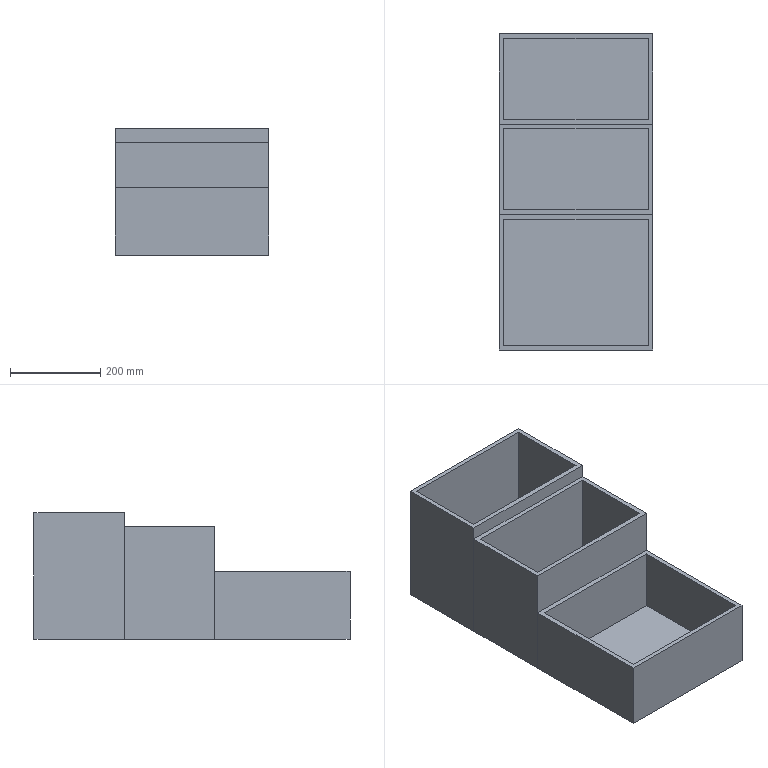Part | SolidWorks | features Shell 3, ICE 2, Extrusion 1 | 3 solids | 33 faces | box 340 x 700 x 280 mm | volume 9420000 mm3 | plane 33
STEP:
#1=CARTESIAN_POINT('',(170.,-100.,280.));
#2=VERTEX_POINT('',#1);
#3=CARTESIAN_POINT('',(170.,100.,280.));
#4=VERTEX_POINT('',#3);
#5=CARTESIAN_POINT('',(170.,-100.,280.));
#6=DIRECTION('',(0.,1.,0.));
#7=VECTOR('',#6,1000.);
#8=LINE('',#5,#7);
#9=EDGE_CURVE('',#2,#4,#8,.T.);
#10=ORIENTED_EDGE('',*,*,#9,.T.);
#11=CARTESIAN_POINT('',(-170.,100.,280.));
#12=VERTEX_POINT('',#11);
#13=CARTESIAN_POINT('',(-170.,100.,280.));
#14=DIRECTION('',(-1.,0.,0.));
#15=VECTOR('',#14,1000.);
#16=LINE('',#13,#15);
#17=EDGE_CURVE('',#4,#12,#16,.T.);
#18=ORIENTED_EDGE('',*,*,#17,.T.);
#19=CARTESIAN_POINT('',(-170.,-100.,280.));
#20=VERTEX_POINT('',#19);
#21=CARTESIAN_POINT('',(-170.,-100.,280.));
#22=DIRECTION('',(0.,-1.,0.));
#23=VECTOR('',#22,1000.);
#24=LINE('',#21,#23);
#25=EDGE_CURVE('',#12,#20,#24,.T.);
#26=ORIENTED_EDGE('',*,*,#25,.T.);
#27=CARTESIAN_POINT('',(-170.,-100.,280.));
#28=DIRECTION('',(1.,0.,0.));
#29=VECTOR('',#28,1000.);
#30=LINE('',#27,#29);
#31=EDGE_CURVE('',#20,#2,#30,.T.);
#32=ORIENTED_EDGE('',*,*,#31,.T.);
#33=EDGE_LOOP('',(#10,#18,#26,#32));
#34=FACE_OUTER_BOUND('',#33,.T.);
#35=CARTESIAN_POINT('',(160.,-90.,280.));
#36=VERTEX_POINT('',#35);
#37=CARTESIAN_POINT('',(160.,90.,280.));
#38=VERTEX_POINT('',#37);
#39=CARTESIAN_POINT('',(160.,0.,280.));
#40=DIRECTION('',(0.,1.,0.));
#41=VECTOR('',#40,1000.);
#42=LINE('',#39,#41);
#43=EDGE_CURVE('',#36,#38,#42,.T.);
#44=ORIENTED_EDGE('',*,*,#43,.F.);
#45=CARTESIAN_POINT('',(-160.,-90.,280.));
#46=VERTEX_POINT('',#45);
#47=CARTESIAN_POINT('',(0.,-90.,280.));
#48=DIRECTION('',(1.,0.,0.));
#49=VECTOR('',#48,1000.);
#50=LINE('',#47,#49);
#51=EDGE_CURVE('',#46,#36,#50,.T.);
#52=ORIENTED_EDGE('',*,*,#51,.F.);
#53=CARTESIAN_POINT('',(-160.,90.,280.));
#54=VERTEX_POINT('',#53);
#55=CARTESIAN_POINT('',(-160.,0.,280.));
#56=DIRECTION('',(0.,-1.,0.));
#57=VECTOR('',#56,1000.);
#58=LINE('',#55,#57);
#59=EDGE_CURVE('',#54,#46,#58,.T.);
#60=ORIENTED_EDGE('',*,*,#59,.F.);
#61=CARTESIAN_POINT('',(0.,90.,280.));
#62=DIRECTION('',(-1.,0.,0.));
#63=VECTOR('',#62,1000.);
#64=LINE('',#61,#63);
#65=EDGE_CURVE('',#38,#54,#64,.T.);
#66=ORIENTED_EDGE('',*,*,#65,.F.);
#67=EDGE_LOOP('',(#44,#52,#60,#66));
#68=FACE_BOUND('',#67,.T.);
#69=CARTESIAN_POINT('',(0.,0.,280.));
#70=DIRECTION('',(0.,0.,-1.));
#71=DIRECTION('',(-1.,0.,0.));
#72=AXIS2_PLACEMENT_3D('',#69,#70,#71);
#73=PLANE('',#72);
#74=ADVANCED_FACE('',(#34,#68),#73,.F.);
#75=CARTESIAN_POINT('',(170.,-100.,0.));
#76=VERTEX_POINT('',#75);
#77=CARTESIAN_POINT('',(170.,100.,0.));
#78=VERTEX_POINT('',#77);
#79=CARTESIAN_POINT('',(170.,-100.,0.));
#80=DIRECTION('',(0.,1.,0.));
#81=VECTOR('',#80,1000.);
#82=LINE('',#79,#81);
#83=EDGE_CURVE('',#76,#78,#82,.T.);
#84=ORIENTED_EDGE('',*,*,#83,.T.);
#85=CARTESIAN_POINT('',(170.,100.,280.));
#86=DIRECTION('',(0.,0.,-1.));
#87=VECTOR('',#86,1000.);
#88=LINE('',#85,#87);
#89=EDGE_CURVE('',#4,#78,#88,.T.);
#90=ORIENTED_EDGE('',*,*,#89,.F.);
#91=ORIENTED_EDGE('',*,*,#9,.F.);
#92=CARTESIAN_POINT('',(170.,-100.,280.));
#93=DIRECTION('',(0.,0.,-1.));
#94=VECTOR('',#93,1000.);
#95=LINE('',#92,#94);
#96=EDGE_CURVE('',#2,#76,#95,.T.);
#97=ORIENTED_EDGE('',*,*,#96,.T.);
#98=EDGE_LOOP('',(#84,#90,#91,#97));
#99=FACE_OUTER_BOUND('',#98,.T.);
#100=CARTESIAN_POINT('',(170.,-100.,280.));
#101=DIRECTION('',(-1.,0.,0.));
#102=DIRECTION('',(0.,0.,1.));
#103=AXIS2_PLACEMENT_3D('',#100,#101,#102);
#104=PLANE('',#103);
#105=ADVANCED_FACE('',(#99),#104,.F.);
#106=CARTESIAN_POINT('',(-170.,100.,0.));
#107=VERTEX_POINT('',#106);
#108=CARTESIAN_POINT('',(-170.,100.,0.));
#109=DIRECTION('',(-1.,0.,0.));
#110=VECTOR('',#109,1000.);
#111=LINE('',#108,#110);
#112=EDGE_CURVE('',#78,#107,#111,.T.);
#113=ORIENTED_EDGE('',*,*,#112,.T.);
#114=CARTESIAN_POINT('',(-170.,100.,280.));
#115=DIRECTION('',(0.,0.,-1.));
#116=VECTOR('',#115,1000.);
#117=LINE('',#114,#116);
#118=EDGE_CURVE('',#12,#107,#117,.T.);
#119=ORIENTED_EDGE('',*,*,#118,.F.);
#120=ORIENTED_EDGE('',*,*,#17,.F.);
#121=ORIENTED_EDGE('',*,*,#89,.T.);
#122=EDGE_LOOP('',(#113,#119,#120,#121));
#123=FACE_OUTER_BOUND('',#122,.T.);
#124=CARTESIAN_POINT('',(-170.,100.,280.));
#125=DIRECTION('',(0.,-1.,0.));
#126=DIRECTION('',(0.,0.,-1.));
#127=AXIS2_PLACEMENT_3D('',#124,#125,#126);
#128=PLANE('',#127);
#129=ADVANCED_FACE('',(#123),#128,.F.);
#130=CARTESIAN_POINT('',(-170.,-100.,0.));
#131=VERTEX_POINT('',#130);
#132=CARTESIAN_POINT('',(-170.,-100.,0.));
#133=DIRECTION('',(0.,-1.,0.));
#134=VECTOR('',#133,1000.);
#135=LINE('',#132,#134);
#136=EDGE_CURVE('',#107,#131,#135,.T.);
#137=ORIENTED_EDGE('',*,*,#136,.T.);
#138=CARTESIAN_POINT('',(-170.,-100.,280.));
#139=DIRECTION('',(0.,0.,-1.));
#140=VECTOR('',#139,1000.);
#141=LINE('',#138,#140);
#142=EDGE_CURVE('',#20,#131,#141,.T.);
#143=ORIENTED_EDGE('',*,*,#142,.F.);
#144=ORIENTED_EDGE('',*,*,#25,.F.);
#145=ORIENTED_EDGE('',*,*,#118,.T.);
#146=EDGE_LOOP('',(#137,#143,#144,#145));
#147=FACE_OUTER_BOUND('',#146,.T.);
#148=CARTESIAN_POINT('',(-170.,-100.,280.));
#149=DIRECTION('',(1.,0.,0.));
#150=DIRECTION('',(0.,0.,-1.));
#151=AXIS2_PLACEMENT_3D('',#148,#149,#150);
#152=PLANE('',#151);
#153=ADVANCED_FACE('',(#147),#152,.F.);
#154=CARTESIAN_POINT('',(-170.,-100.,0.));
#155=DIRECTION('',(1.,0.,0.));
#156=VECTOR('',#155,1000.);
#157=LINE('',#154,#156);
#158=EDGE_CURVE('',#131,#76,#157,.T.);
#159=ORIENTED_EDGE('',*,*,#158,.T.);
#160=ORIENTED_EDGE('',*,*,#96,.F.);
#161=ORIENTED_EDGE('',*,*,#31,.F.);
#162=ORIENTED_EDGE('',*,*,#142,.T.);
#163=EDGE_LOOP('',(#159,#160,#161,#162));
#164=FACE_OUTER_BOUND('',#163,.T.);
#165=CARTESIAN_POINT('',(-170.,-100.,280.));
#166=DIRECTION('',(0.,1.,0.));
#167=DIRECTION('',(0.,0.,1.));
#168=AXIS2_PLACEMENT_3D('',#165,#166,#167);
#169=PLANE('',#168);
#170=ADVANCED_FACE('',(#164),#169,.F.);
#171=ORIENTED_EDGE('',*,*,#83,.F.);
#172=ORIENTED_EDGE('',*,*,#158,.F.);
#173=ORIENTED_EDGE('',*,*,#136,.F.);
#174=ORIENTED_EDGE('',*,*,#112,.F.);
#175=EDGE_LOOP('',(#171,#172,#173,#174));
#176=FACE_OUTER_BOUND('',#175,.T.);
#177=CARTESIAN_POINT('',(0.,0.,0.));
#178=DIRECTION('',(0.,0.,-1.));
#179=DIRECTION('',(-1.,0.,0.));
#180=AXIS2_PLACEMENT_3D('',#177,#178,#179);
#181=PLANE('',#180);
#182=ADVANCED_FACE('',(#176),#181,.T.);
#183=CARTESIAN_POINT('',(160.,-90.,10.));
#184=VERTEX_POINT('',#183);
#185=CARTESIAN_POINT('',(160.,90.,10.));
#186=VERTEX_POINT('',#185);
#187=CARTESIAN_POINT('',(160.,0.,10.));
#188=DIRECTION('',(0.,1.,0.));
#189=VECTOR('',#188,1000.);
#190=LINE('',#187,#189);
#191=EDGE_CURVE('',#184,#186,#190,.T.);
#192=ORIENTED_EDGE('',*,*,#191,.F.);
#193=CARTESIAN_POINT('',(160.,-90.,280.));
#194=DIRECTION('',(0.,0.,-1.));
#195=VECTOR('',#194,1000.);
#196=LINE('',#193,#195);
#197=EDGE_CURVE('',#36,#184,#196,.T.);
#198=ORIENTED_EDGE('',*,*,#197,.F.);
#199=ORIENTED_EDGE('',*,*,#43,.T.);
#200=CARTESIAN_POINT('',(160.,90.,280.));
#201=DIRECTION('',(0.,0.,-1.));
#202=VECTOR('',#201,1000.);
#203=LINE('',#200,#202);
#204=EDGE_CURVE('',#38,#186,#203,.T.);
#205=ORIENTED_EDGE('',*,*,#204,.T.);
#206=EDGE_LOOP('',(#192,#198,#199,#205));
#207=FACE_OUTER_BOUND('',#206,.T.);
#208=CARTESIAN_POINT('',(160.,-100.,280.));
#209=DIRECTION('',(-1.,0.,0.));
#210=DIRECTION('',(0.,0.,1.));
#211=AXIS2_PLACEMENT_3D('',#208,#209,#210);
#212=PLANE('',#211);
#213=ADVANCED_FACE('',(#207),#212,.T.);
#214=CARTESIAN_POINT('',(-160.,90.,10.));
#215=VERTEX_POINT('',#214);
#216=CARTESIAN_POINT('',(0.,90.,10.));
#217=DIRECTION('',(-1.,0.,0.));
#218=VECTOR('',#217,1000.);
#219=LINE('',#216,#218);
#220=EDGE_CURVE('',#186,#215,#219,.T.);
#221=ORIENTED_EDGE('',*,*,#220,.F.);
#222=ORIENTED_EDGE('',*,*,#204,.F.);
#223=ORIENTED_EDGE('',*,*,#65,.T.);
#224=CARTESIAN_POINT('',(-160.,90.,280.));
#225=DIRECTION('',(0.,0.,-1.));
#226=VECTOR('',#225,1000.);
#227=LINE('',#224,#226);
#228=EDGE_CURVE('',#54,#215,#227,.T.);
#229=ORIENTED_EDGE('',*,*,#228,.T.);
#230=EDGE_LOOP('',(#221,#222,#223,#229));
#231=FACE_OUTER_BOUND('',#230,.T.);
#232=CARTESIAN_POINT('',(-170.,90.,280.));
#233=DIRECTION('',(0.,-1.,0.));
#234=DIRECTION('',(0.,0.,-1.));
#235=AXIS2_PLACEMENT_3D('',#232,#233,#234);
#236=PLANE('',#235);
#237=ADVANCED_FACE('',(#231),#236,.T.);
#238=CARTESIAN_POINT('',(-160.,-90.,10.));
#239=VERTEX_POINT('',#238);
#240=CARTESIAN_POINT('',(-160.,0.,10.));
#241=DIRECTION('',(0.,-1.,0.));
#242=VECTOR('',#241,1000.);
#243=LINE('',#240,#242);
#244=EDGE_CURVE('',#215,#239,#243,.T.);
#245=ORIENTED_EDGE('',*,*,#244,.F.);
#246=ORIENTED_EDGE('',*,*,#228,.F.);
#247=ORIENTED_EDGE('',*,*,#59,.T.);
#248=CARTESIAN_POINT('',(-160.,-90.,280.));
#249=DIRECTION('',(0.,0.,-1.));
#250=VECTOR('',#249,1000.);
#251=LINE('',#248,#250);
#252=EDGE_CURVE('',#46,#239,#251,.T.);
#253=ORIENTED_EDGE('',*,*,#252,.T.);
#254=EDGE_LOOP('',(#245,#246,#247,#253));
#255=FACE_OUTER_BOUND('',#254,.T.);
#256=CARTESIAN_POINT('',(-160.,-100.,280.));
#257=DIRECTION('',(1.,0.,0.));
#258=DIRECTION('',(0.,0.,-1.));
#259=AXIS2_PLACEMENT_3D('',#256,#257,#258);
#260=PLANE('',#259);
#261=ADVANCED_FACE('',(#255),#260,.T.);
#262=CARTESIAN_POINT('',(0.,-90.,10.));
#263=DIRECTION('',(1.,0.,0.));
#264=VECTOR('',#263,1000.);
#265=LINE('',#262,#264);
#266=EDGE_CURVE('',#239,#184,#265,.T.);
#267=ORIENTED_EDGE('',*,*,#266,.F.);
#268=ORIENTED_EDGE('',*,*,#252,.F.);
#269=ORIENTED_EDGE('',*,*,#51,.T.);
#270=ORIENTED_EDGE('',*,*,#197,.T.);
#271=EDGE_LOOP('',(#267,#268,#269,#270));
#272=FACE_OUTER_BOUND('',#271,.T.);
#273=CARTESIAN_POINT('',(-170.,-90.,280.));
#274=DIRECTION('',(0.,1.,0.));
#275=DIRECTION('',(0.,0.,1.));
#276=AXIS2_PLACEMENT_3D('',#273,#274,#275);
#277=PLANE('',#276);
#278=ADVANCED_FACE('',(#272),#277,.T.);
#279=ORIENTED_EDGE('',*,*,#191,.T.);
#280=ORIENTED_EDGE('',*,*,#220,.T.);
#281=ORIENTED_EDGE('',*,*,#244,.T.);
#282=ORIENTED_EDGE('',*,*,#266,.T.);
#283=EDGE_LOOP('',(#279,#280,#281,#282));
#284=FACE_OUTER_BOUND('',#283,.T.);
#285=CARTESIAN_POINT('',(0.,0.,10.));
#286=DIRECTION('',(0.,0.,-1.));
#287=DIRECTION('',(-1.,0.,0.));
#288=AXIS2_PLACEMENT_3D('',#285,#286,#287);
#289=PLANE('',#288);
#290=ADVANCED_FACE('',(#284),#289,.F.);
#291=CLOSED_SHELL('',(#74,#105,#129,#153,#170,#182,#213,#237,#261,#278,#290));
#292=MANIFOLD_SOLID_BREP('',#291);
#293=CARTESIAN_POINT('',(170.,-100.,0.));
#294=VERTEX_POINT('',#293);
#295=CARTESIAN_POINT('',(170.,-300.,0.));
#296=VERTEX_POINT('',#295);
#297=CARTESIAN_POINT('',(170.,-100.,0.));
#298=DIRECTION('',(0.,-1.,0.));
#299=VECTOR('',#298,1000.);
#300=LINE('',#297,#299);
#301=EDGE_CURVE('',#294,#296,#300,.T.);
#302=ORIENTED_EDGE('',*,*,#301,.F.);
#303=CARTESIAN_POINT('',(170.,-100.,250.));
#304=VERTEX_POINT('',#303);
#305=CARTESIAN_POINT('',(170.,-100.,250.));
#306=DIRECTION('',(0.,0.,-1.));
#307=VECTOR('',#306,1000.);
#308=LINE('',#305,#307);
#309=EDGE_CURVE('',#304,#294,#308,.T.);
#310=ORIENTED_EDGE('',*,*,#309,.F.);
#311=CARTESIAN_POINT('',(170.,-300.,250.));
#312=VERTEX_POINT('',#311);
#313=CARTESIAN_POINT('',(170.,-100.,250.));
#314=DIRECTION('',(0.,-1.,0.));
#315=VECTOR('',#314,1000.);
#316=LINE('',#313,#315);
#317=EDGE_CURVE('',#304,#312,#316,.T.);
#318=ORIENTED_EDGE('',*,*,#317,.T.);
#319=CARTESIAN_POINT('',(170.,-300.,250.));
#320=DIRECTION('',(0.,0.,-1.));
#321=VECTOR('',#320,1000.);
#322=LINE('',#319,#321);
#323=EDGE_CURVE('',#312,#296,#322,.T.);
#324=ORIENTED_EDGE('',*,*,#323,.T.);
#325=EDGE_LOOP('',(#302,#310,#318,#324));
#326=FACE_OUTER_BOUND('',#325,.T.);
#327=CARTESIAN_POINT('',(170.,-100.,250.));
#328=DIRECTION('',(1.,0.,0.));
#329=DIRECTION('',(0.,1.,0.));
#330=AXIS2_PLACEMENT_3D('',#327,#328,#329);
#331=PLANE('',#330);
#332=ADVANCED_FACE('',(#326),#331,.T.);
#333=CARTESIAN_POINT('',(-170.,-100.,0.));
#334=VERTEX_POINT('',#333);
#335=CARTESIAN_POINT('',(170.,-100.,0.));
#336=DIRECTION('',(1.,0.,0.));
#337=VECTOR('',#336,1000.);
#338=LINE('',#335,#337);
#339=EDGE_CURVE('',#334,#294,#338,.T.);
#340=ORIENTED_EDGE('',*,*,#339,.F.);
#341=CARTESIAN_POINT('',(-170.,-100.,250.));
#342=VERTEX_POINT('',#341);
#343=CARTESIAN_POINT('',(-170.,-100.,250.));
#344=DIRECTION('',(0.,0.,-1.));
#345=VECTOR('',#344,1000.);
#346=LINE('',#343,#345);
#347=EDGE_CURVE('',#342,#334,#346,.T.);
#348=ORIENTED_EDGE('',*,*,#347,.F.);
#349=CARTESIAN_POINT('',(170.,-100.,250.));
#350=DIRECTION('',(1.,0.,0.));
#351=VECTOR('',#350,1000.);
#352=LINE('',#349,#351);
#353=EDGE_CURVE('',#342,#304,#352,.T.);
#354=ORIENTED_EDGE('',*,*,#353,.T.);
#355=ORIENTED_EDGE('',*,*,#309,.T.);
#356=EDGE_LOOP('',(#340,#348,#354,#355));
#357=FACE_OUTER_BOUND('',#356,.T.);
#358=CARTESIAN_POINT('',(170.,-100.,250.));
#359=DIRECTION('',(0.,1.,0.));
#360=DIRECTION('',(0.,0.,1.));
#361=AXIS2_PLACEMENT_3D('',#358,#359,#360);
#362=PLANE('',#361);
#363=ADVANCED_FACE('',(#357),#362,.T.);
#364=CARTESIAN_POINT('',(-170.,-300.,0.));
#365=VERTEX_POINT('',#364);
#366=CARTESIAN_POINT('',(-170.,-100.,0.));
#367=DIRECTION('',(0.,1.,0.));
#368=VECTOR('',#367,1000.);
#369=LINE('',#366,#368);
#370=EDGE_CURVE('',#365,#334,#369,.T.);
#371=ORIENTED_EDGE('',*,*,#370,.F.);
#372=CARTESIAN_POINT('',(-170.,-300.,250.));
#373=VERTEX_POINT('',#372);
#374=CARTESIAN_POINT('',(-170.,-300.,250.));
#375=DIRECTION('',(0.,0.,-1.));
#376=VECTOR('',#375,1000.);
#377=LINE('',#374,#376);
#378=EDGE_CURVE('',#373,#365,#377,.T.);
#379=ORIENTED_EDGE('',*,*,#378,.F.);
#380=CARTESIAN_POINT('',(-170.,-100.,250.));
#381=DIRECTION('',(0.,1.,0.));
#382=VECTOR('',#381,1000.);
#383=LINE('',#380,#382);
#384=EDGE_CURVE('',#373,#342,#383,.T.);
#385=ORIENTED_EDGE('',*,*,#384,.T.);
#386=ORIENTED_EDGE('',*,*,#347,.T.);
#387=EDGE_LOOP('',(#371,#379,#385,#386));
#388=FACE_OUTER_BOUND('',#387,.T.);
#389=CARTESIAN_POINT('',(-170.,-100.,250.));
#390=DIRECTION('',(-1.,0.,0.));
#391=DIRECTION('',(0.,-1.,0.));
#392=AXIS2_PLACEMENT_3D('',#389,#390,#391);
#393=PLANE('',#392);
#394=ADVANCED_FACE('',(#388),#393,.T.);
#395=CARTESIAN_POINT('',(170.,-300.,0.));
#396=DIRECTION('',(-1.,0.,0.));
#397=VECTOR('',#396,1000.);
#398=LINE('',#395,#397);
#399=EDGE_CURVE('',#296,#365,#398,.T.);
#400=ORIENTED_EDGE('',*,*,#399,.F.);
#401=ORIENTED_EDGE('',*,*,#323,.F.);
#402=CARTESIAN_POINT('',(170.,-300.,250.));
#403=DIRECTION('',(-1.,0.,0.));
#404=VECTOR('',#403,1000.);
#405=LINE('',#402,#404);
#406=EDGE_CURVE('',#312,#373,#405,.T.);
#407=ORIENTED_EDGE('',*,*,#406,.T.);
#408=ORIENTED_EDGE('',*,*,#378,.T.);
#409=EDGE_LOOP('',(#400,#401,#407,#408));
#410=FACE_OUTER_BOUND('',#409,.T.);
#411=CARTESIAN_POINT('',(170.,-300.,250.));
#412=DIRECTION('',(0.,-1.,0.));
#413=DIRECTION('',(0.,0.,-1.));
#414=AXIS2_PLACEMENT_3D('',#411,#412,#413);
#415=PLANE('',#414);
#416=ADVANCED_FACE('',(#410),#415,.T.);
#417=CARTESIAN_POINT('',(-160.,-110.,250.));
#418=VERTEX_POINT('',#417);
#419=CARTESIAN_POINT('',(160.,-110.,250.));
#420=VERTEX_POINT('',#419);
#421=CARTESIAN_POINT('',(0.,-110.,250.));
#422=DIRECTION('',(1.,0.,0.));
#423=VECTOR('',#422,1000.);
#424=LINE('',#421,#423);
#425=EDGE_CURVE('',#418,#420,#424,.T.);
#426=ORIENTED_EDGE('',*,*,#425,.T.);
#427=CARTESIAN_POINT('',(160.,-290.,250.));
#428=VERTEX_POINT('',#427);
#429=CARTESIAN_POINT('',(160.,0.,250.));
#430=DIRECTION('',(0.,-1.,0.));
#431=VECTOR('',#430,1000.);
#432=LINE('',#429,#431);
#433=EDGE_CURVE('',#420,#428,#432,.T.);
#434=ORIENTED_EDGE('',*,*,#433,.T.);
#435=CARTESIAN_POINT('',(-160.,-290.,250.));
#436=VERTEX_POINT('',#435);
#437=CARTESIAN_POINT('',(0.,-290.,250.));
#438=DIRECTION('',(-1.,0.,0.));
#439=VECTOR('',#438,1000.);
#440=LINE('',#437,#439);
#441=EDGE_CURVE('',#428,#436,#440,.T.);
#442=ORIENTED_EDGE('',*,*,#441,.T.);
#443=CARTESIAN_POINT('',(-160.,0.,250.));
#444=DIRECTION('',(0.,1.,0.));
#445=VECTOR('',#444,1000.);
#446=LINE('',#443,#445);
#447=EDGE_CURVE('',#436,#418,#446,.T.);
#448=ORIENTED_EDGE('',*,*,#447,.T.);
#449=EDGE_LOOP('',(#426,#434,#442,#448));
#450=FACE_BOUND('',#449,.T.);
#451=ORIENTED_EDGE('',*,*,#317,.F.);
#452=ORIENTED_EDGE('',*,*,#353,.F.);
#453=ORIENTED_EDGE('',*,*,#384,.F.);
#454=ORIENTED_EDGE('',*,*,#406,.F.);
#455=EDGE_LOOP('',(#451,#452,#453,#454));
#456=FACE_OUTER_BOUND('',#455,.T.);
#457=CARTESIAN_POINT('',(0.,0.,250.));
#458=DIRECTION('',(0.,0.,-1.));
#459=DIRECTION('',(-1.,0.,0.));
#460=AXIS2_PLACEMENT_3D('',#457,#458,#459);
#461=PLANE('',#460);
#462=ADVANCED_FACE('',(#450,#456),#461,.F.);
#463=ORIENTED_EDGE('',*,*,#301,.T.);
#464=ORIENTED_EDGE('',*,*,#399,.T.);
#465=ORIENTED_EDGE('',*,*,#370,.T.);
#466=ORIENTED_EDGE('',*,*,#339,.T.);
#467=EDGE_LOOP('',(#463,#464,#465,#466));
#468=FACE_OUTER_BOUND('',#467,.T.);
#469=CARTESIAN_POINT('',(0.,0.,0.));
#470=DIRECTION('',(0.,0.,-1.));
#471=DIRECTION('',(-1.,0.,0.));
#472=AXIS2_PLACEMENT_3D('',#469,#470,#471);
#473=PLANE('',#472);
#474=ADVANCED_FACE('',(#468),#473,.T.);
#475=CARTESIAN_POINT('',(160.,-110.,10.));
#476=VERTEX_POINT('',#475);
#477=CARTESIAN_POINT('',(160.,-290.,10.));
#478=VERTEX_POINT('',#477);
#479=CARTESIAN_POINT('',(160.,0.,10.));
#480=DIRECTION('',(0.,-1.,0.));
#481=VECTOR('',#480,1000.);
#482=LINE('',#479,#481);
#483=EDGE_CURVE('',#476,#478,#482,.T.);
#484=ORIENTED_EDGE('',*,*,#483,.T.);
#485=CARTESIAN_POINT('',(160.,-290.,250.));
#486=DIRECTION('',(0.,0.,-1.));
#487=VECTOR('',#486,1000.);
#488=LINE('',#485,#487);
#489=EDGE_CURVE('',#428,#478,#488,.T.);
#490=ORIENTED_EDGE('',*,*,#489,.F.);
#491=ORIENTED_EDGE('',*,*,#433,.F.);
#492=CARTESIAN_POINT('',(160.,-110.,250.));
#493=DIRECTION('',(0.,0.,-1.));
#494=VECTOR('',#493,1000.);
#495=LINE('',#492,#494);
#496=EDGE_CURVE('',#420,#476,#495,.T.);
#497=ORIENTED_EDGE('',*,*,#496,.T.);
#498=EDGE_LOOP('',(#484,#490,#491,#497));
#499=FACE_OUTER_BOUND('',#498,.T.);
#500=CARTESIAN_POINT('',(160.,-100.,250.));
#501=DIRECTION('',(1.,0.,0.));
#502=DIRECTION('',(0.,1.,0.));
#503=AXIS2_PLACEMENT_3D('',#500,#501,#502);
#504=PLANE('',#503);
#505=ADVANCED_FACE('',(#499),#504,.F.);
#506=CARTESIAN_POINT('',(-160.,-110.,10.));
#507=VERTEX_POINT('',#506);
#508=CARTESIAN_POINT('',(0.,-110.,10.));
#509=DIRECTION('',(1.,0.,0.));
#510=VECTOR('',#509,1000.);
#511=LINE('',#508,#510);
#512=EDGE_CURVE('',#507,#476,#511,.T.);
#513=ORIENTED_EDGE('',*,*,#512,.T.);
#514=ORIENTED_EDGE('',*,*,#496,.F.);
#515=ORIENTED_EDGE('',*,*,#425,.F.);
#516=CARTESIAN_POINT('',(-160.,-110.,250.));
#517=DIRECTION('',(0.,0.,-1.));
#518=VECTOR('',#517,1000.);
#519=LINE('',#516,#518);
#520=EDGE_CURVE('',#418,#507,#519,.T.);
#521=ORIENTED_EDGE('',*,*,#520,.T.);
#522=EDGE_LOOP('',(#513,#514,#515,#521));
#523=FACE_OUTER_BOUND('',#522,.T.);
#524=CARTESIAN_POINT('',(170.,-110.,250.));
#525=DIRECTION('',(0.,1.,0.));
#526=DIRECTION('',(0.,0.,1.));
#527=AXIS2_PLACEMENT_3D('',#524,#525,#526);
#528=PLANE('',#527);
#529=ADVANCED_FACE('',(#523),#528,.F.);
#530=CARTESIAN_POINT('',(-160.,-290.,10.));
#531=VERTEX_POINT('',#530);
#532=CARTESIAN_POINT('',(-160.,0.,10.));
#533=DIRECTION('',(0.,1.,0.));
#534=VECTOR('',#533,1000.);
#535=LINE('',#532,#534);
#536=EDGE_CURVE('',#531,#507,#535,.T.);
#537=ORIENTED_EDGE('',*,*,#536,.T.);
#538=ORIENTED_EDGE('',*,*,#520,.F.);
#539=ORIENTED_EDGE('',*,*,#447,.F.);
#540=CARTESIAN_POINT('',(-160.,-290.,250.));
#541=DIRECTION('',(0.,0.,-1.));
#542=VECTOR('',#541,1000.);
#543=LINE('',#540,#542);
#544=EDGE_CURVE('',#436,#531,#543,.T.);
#545=ORIENTED_EDGE('',*,*,#544,.T.);
#546=EDGE_LOOP('',(#537,#538,#539,#545));
#547=FACE_OUTER_BOUND('',#546,.T.);
#548=CARTESIAN_POINT('',(-160.,-100.,250.));
#549=DIRECTION('',(-1.,0.,0.));
#550=DIRECTION('',(0.,-1.,0.));
#551=AXIS2_PLACEMENT_3D('',#548,#549,#550);
#552=PLANE('',#551);
#553=ADVANCED_FACE('',(#547),#552,.F.);
#554=CARTESIAN_POINT('',(0.,-290.,10.));
#555=DIRECTION('',(-1.,0.,0.));
#556=VECTOR('',#555,1000.);
#557=LINE('',#554,#556);
#558=EDGE_CURVE('',#478,#531,#557,.T.);
#559=ORIENTED_EDGE('',*,*,#558,.T.);
#560=ORIENTED_EDGE('',*,*,#544,.F.);
#561=ORIENTED_EDGE('',*,*,#441,.F.);
#562=ORIENTED_EDGE('',*,*,#489,.T.);
#563=EDGE_LOOP('',(#559,#560,#561,#562));
#564=FACE_OUTER_BOUND('',#563,.T.);
#565=CARTESIAN_POINT('',(170.,-290.,250.));
#566=DIRECTION('',(0.,-1.,0.));
#567=DIRECTION('',(0.,0.,-1.));
#568=AXIS2_PLACEMENT_3D('',#565,#566,#567);
#569=PLANE('',#568);
#570=ADVANCED_FACE('',(#564),#569,.F.);
#571=ORIENTED_EDGE('',*,*,#483,.F.);
#572=ORIENTED_EDGE('',*,*,#512,.F.);
#573=ORIENTED_EDGE('',*,*,#536,.F.);
#574=ORIENTED_EDGE('',*,*,#558,.F.);
#575=EDGE_LOOP('',(#571,#572,#573,#574));
#576=FACE_OUTER_BOUND('',#575,.T.);
#577=CARTESIAN_POINT('',(0.,0.,10.));
#578=DIRECTION('',(0.,0.,-1.));
#579=DIRECTION('',(-1.,0.,0.));
#580=AXIS2_PLACEMENT_3D('',#577,#578,#579);
#581=PLANE('',#580);
#582=ADVANCED_FACE('',(#576),#581,.F.);
#583=CLOSED_SHELL('',(#332,#363,#394,#416,#462,#474,#505,#529,#553,#570,#582));
#584=MANIFOLD_SOLID_BREP('',#583);
#585=CARTESIAN_POINT('',(170.,-300.,0.));
#586=VERTEX_POINT('',#585);
#587=CARTESIAN_POINT('',(170.,-600.,0.));
#588=VERTEX_POINT('',#587);
#589=CARTESIAN_POINT('',(170.,-300.,0.));
#590=DIRECTION('',(0.,-1.,0.));
#591=VECTOR('',#590,1000.);
#592=LINE('',#589,#591);
#593=EDGE_CURVE('',#586,#588,#592,.T.);
#594=ORIENTED_EDGE('',*,*,#593,.F.);
#595=CARTESIAN_POINT('',(170.,-300.,150.));
#596=VERTEX_POINT('',#595);
#597=CARTESIAN_POINT('',(170.,-300.,150.));
#598=DIRECTION('',(0.,0.,-1.));
#599=VECTOR('',#598,1000.);
#600=LINE('',#597,#599);
#601=EDGE_CURVE('',#596,#586,#600,.T.);
#602=ORIENTED_EDGE('',*,*,#601,.F.);
#603=CARTESIAN_POINT('',(170.,-600.,150.));
#604=VERTEX_POINT('',#603);
#605=CARTESIAN_POINT('',(170.,-300.,150.));
#606=DIRECTION('',(0.,-1.,0.));
#607=VECTOR('',#606,1000.);
#608=LINE('',#605,#607);
#609=EDGE_CURVE('',#596,#604,#608,.T.);
#610=ORIENTED_EDGE('',*,*,#609,.T.);
#611=CARTESIAN_POINT('',(170.,-600.,150.));
#612=DIRECTION('',(0.,0.,-1.));
#613=VECTOR('',#612,1000.);
#614=LINE('',#611,#613);
#615=EDGE_CURVE('',#604,#588,#614,.T.);
#616=ORIENTED_EDGE('',*,*,#615,.T.);
#617=EDGE_LOOP('',(#594,#602,#610,#616));
#618=FACE_OUTER_BOUND('',#617,.T.);
#619=CARTESIAN_POINT('',(170.,-300.,150.));
#620=DIRECTION('',(1.,0.,0.));
#621=DIRECTION('',(0.,1.,0.));
#622=AXIS2_PLACEMENT_3D('',#619,#620,#621);
#623=PLANE('',#622);
#624=ADVANCED_FACE('',(#618),#623,.T.);
#625=CARTESIAN_POINT('',(-170.,-300.,0.));
#626=VERTEX_POINT('',#625);
#627=CARTESIAN_POINT('',(170.,-300.,0.));
#628=DIRECTION('',(1.,0.,0.));
#629=VECTOR('',#628,1000.);
#630=LINE('',#627,#629);
#631=EDGE_CURVE('',#626,#586,#630,.T.);
#632=ORIENTED_EDGE('',*,*,#631,.F.);
#633=CARTESIAN_POINT('',(-170.,-300.,150.));
#634=VERTEX_POINT('',#633);
#635=CARTESIAN_POINT('',(-170.,-300.,150.));
#636=DIRECTION('',(0.,0.,-1.));
#637=VECTOR('',#636,1000.);
#638=LINE('',#635,#637);
#639=EDGE_CURVE('',#634,#626,#638,.T.);
#640=ORIENTED_EDGE('',*,*,#639,.F.);
#641=CARTESIAN_POINT('',(170.,-300.,150.));
#642=DIRECTION('',(1.,0.,0.));
#643=VECTOR('',#642,1000.);
#644=LINE('',#641,#643);
#645=EDGE_CURVE('',#634,#596,#644,.T.);
#646=ORIENTED_EDGE('',*,*,#645,.T.);
#647=ORIENTED_EDGE('',*,*,#601,.T.);
#648=EDGE_LOOP('',(#632,#640,#646,#647));
#649=FACE_OUTER_BOUND('',#648,.T.);
#650=CARTESIAN_POINT('',(170.,-300.,150.));
#651=DIRECTION('',(0.,1.,0.));
#652=DIRECTION('',(0.,0.,1.));
#653=AXIS2_PLACEMENT_3D('',#650,#651,#652);
#654=PLANE('',#653);
#655=ADVANCED_FACE('',(#649),#654,.T.);
#656=CARTESIAN_POINT('',(-170.,-600.,0.));
#657=VERTEX_POINT('',#656);
#658=CARTESIAN_POINT('',(-170.,-300.,0.));
#659=DIRECTION('',(0.,1.,0.));
#660=VECTOR('',#659,1000.);
#661=LINE('',#658,#660);
#662=EDGE_CURVE('',#657,#626,#661,.T.);
#663=ORIENTED_EDGE('',*,*,#662,.F.);
#664=CARTESIAN_POINT('',(-170.,-600.,150.));
#665=VERTEX_POINT('',#664);
#666=CARTESIAN_POINT('',(-170.,-600.,150.));
#667=DIRECTION('',(0.,0.,-1.));
#668=VECTOR('',#667,1000.);
#669=LINE('',#666,#668);
#670=EDGE_CURVE('',#665,#657,#669,.T.);
#671=ORIENTED_EDGE('',*,*,#670,.F.);
#672=CARTESIAN_POINT('',(-170.,-300.,150.));
#673=DIRECTION('',(0.,1.,0.));
#674=VECTOR('',#673,1000.);
#675=LINE('',#672,#674);
#676=EDGE_CURVE('',#665,#634,#675,.T.);
#677=ORIENTED_EDGE('',*,*,#676,.T.);
#678=ORIENTED_EDGE('',*,*,#639,.T.);
#679=EDGE_LOOP('',(#663,#671,#677,#678));
#680=FACE_OUTER_BOUND('',#679,.T.);
#681=CARTESIAN_POINT('',(-170.,-300.,150.));
#682=DIRECTION('',(-1.,0.,0.));
#683=DIRECTION('',(0.,0.,1.));
#684=AXIS2_PLACEMENT_3D('',#681,#682,#683);
#685=PLANE('',#684);
#686=ADVANCED_FACE('',(#680),#685,.T.);
#687=CARTESIAN_POINT('',(170.,-600.,0.));
#688=DIRECTION('',(-1.,0.,0.));
#689=VECTOR('',#688,1000.);
#690=LINE('',#687,#689);
#691=EDGE_CURVE('',#588,#657,#690,.T.);
#692=ORIENTED_EDGE('',*,*,#691,.F.);
#693=ORIENTED_EDGE('',*,*,#615,.F.);
#694=CARTESIAN_POINT('',(170.,-600.,150.));
#695=DIRECTION('',(-1.,0.,0.));
#696=VECTOR('',#695,1000.);
#697=LINE('',#694,#696);
#698=EDGE_CURVE('',#604,#665,#697,.T.);
#699=ORIENTED_EDGE('',*,*,#698,.T.);
#700=ORIENTED_EDGE('',*,*,#670,.T.);
#701=EDGE_LOOP('',(#692,#693,#699,#700));
#702=FACE_OUTER_BOUND('',#701,.T.);
#703=CARTESIAN_POINT('',(170.,-600.,150.));
#704=DIRECTION('',(0.,-1.,0.));
#705=DIRECTION('',(0.,0.,-1.));
#706=AXIS2_PLACEMENT_3D('',#703,#704,#705);
#707=PLANE('',#706);
#708=ADVANCED_FACE('',(#702),#707,.T.);
#709=CARTESIAN_POINT('',(-160.,-310.,150.));
#710=VERTEX_POINT('',#709);
#711=CARTESIAN_POINT('',(160.,-310.,150.));
#712=VERTEX_POINT('',#711);
#713=CARTESIAN_POINT('',(0.,-310.,150.));
#714=DIRECTION('',(1.,0.,0.));
#715=VECTOR('',#714,1000.);
#716=LINE('',#713,#715);
#717=EDGE_CURVE('',#710,#712,#716,.T.);
#718=ORIENTED_EDGE('',*,*,#717,.T.);
#719=CARTESIAN_POINT('',(160.,-590.,150.));
#720=VERTEX_POINT('',#719);
#721=CARTESIAN_POINT('',(160.,0.,150.));
#722=DIRECTION('',(0.,-1.,0.));
#723=VECTOR('',#722,1000.);
#724=LINE('',#721,#723);
#725=EDGE_CURVE('',#712,#720,#724,.T.);
#726=ORIENTED_EDGE('',*,*,#725,.T.);
#727=CARTESIAN_POINT('',(-160.,-590.,150.));
#728=VERTEX_POINT('',#727);
#729=CARTESIAN_POINT('',(0.,-590.,150.));
#730=DIRECTION('',(-1.,0.,0.));
#731=VECTOR('',#730,1000.);
#732=LINE('',#729,#731);
#733=EDGE_CURVE('',#720,#728,#732,.T.);
#734=ORIENTED_EDGE('',*,*,#733,.T.);
#735=CARTESIAN_POINT('',(-160.,0.,150.));
#736=DIRECTION('',(0.,1.,0.));
#737=VECTOR('',#736,1000.);
#738=LINE('',#735,#737);
#739=EDGE_CURVE('',#728,#710,#738,.T.);
#740=ORIENTED_EDGE('',*,*,#739,.T.);
#741=EDGE_LOOP('',(#718,#726,#734,#740));
#742=FACE_BOUND('',#741,.T.);
#743=ORIENTED_EDGE('',*,*,#609,.F.);
#744=ORIENTED_EDGE('',*,*,#645,.F.);
#745=ORIENTED_EDGE('',*,*,#676,.F.);
#746=ORIENTED_EDGE('',*,*,#698,.F.);
#747=EDGE_LOOP('',(#743,#744,#745,#746));
#748=FACE_OUTER_BOUND('',#747,.T.);
#749=CARTESIAN_POINT('',(0.,0.,150.));
#750=DIRECTION('',(0.,0.,-1.));
#751=DIRECTION('',(-1.,0.,0.));
#752=AXIS2_PLACEMENT_3D('',#749,#750,#751);
#753=PLANE('',#752);
#754=ADVANCED_FACE('',(#742,#748),#753,.F.);
#755=ORIENTED_EDGE('',*,*,#593,.T.);
#756=ORIENTED_EDGE('',*,*,#691,.T.);
#757=ORIENTED_EDGE('',*,*,#662,.T.);
#758=ORIENTED_EDGE('',*,*,#631,.T.);
#759=EDGE_LOOP('',(#755,#756,#757,#758));
#760=FACE_OUTER_BOUND('',#759,.T.);
#761=CARTESIAN_POINT('',(0.,0.,0.));
#762=DIRECTION('',(0.,0.,-1.));
#763=DIRECTION('',(-1.,0.,0.));
#764=AXIS2_PLACEMENT_3D('',#761,#762,#763);
#765=PLANE('',#764);
#766=ADVANCED_FACE('',(#760),#765,.T.);
#767=CARTESIAN_POINT('',(160.,-310.,10.));
#768=VERTEX_POINT('',#767);
#769=CARTESIAN_POINT('',(160.,-590.,10.));
#770=VERTEX_POINT('',#769);
#771=CARTESIAN_POINT('',(160.,0.,10.));
#772=DIRECTION('',(0.,-1.,0.));
#773=VECTOR('',#772,1000.);
#774=LINE('',#771,#773);
#775=EDGE_CURVE('',#768,#770,#774,.T.);
#776=ORIENTED_EDGE('',*,*,#775,.T.);
#777=CARTESIAN_POINT('',(160.,-590.,150.));
#778=DIRECTION('',(0.,0.,-1.));
#779=VECTOR('',#778,1000.);
#780=LINE('',#777,#779);
#781=EDGE_CURVE('',#720,#770,#780,.T.);
#782=ORIENTED_EDGE('',*,*,#781,.F.);
#783=ORIENTED_EDGE('',*,*,#725,.F.);
#784=CARTESIAN_POINT('',(160.,-310.,150.));
#785=DIRECTION('',(0.,0.,-1.));
#786=VECTOR('',#785,1000.);
#787=LINE('',#784,#786);
#788=EDGE_CURVE('',#712,#768,#787,.T.);
#789=ORIENTED_EDGE('',*,*,#788,.T.);
#790=EDGE_LOOP('',(#776,#782,#783,#789));
#791=FACE_OUTER_BOUND('',#790,.T.);
#792=CARTESIAN_POINT('',(160.,-300.,150.));
#793=DIRECTION('',(1.,0.,0.));
#794=DIRECTION('',(0.,1.,0.));
#795=AXIS2_PLACEMENT_3D('',#792,#793,#794);
#796=PLANE('',#795);
#797=ADVANCED_FACE('',(#791),#796,.F.);
#798=CARTESIAN_POINT('',(-160.,-310.,10.));
#799=VERTEX_POINT('',#798);
#800=CARTESIAN_POINT('',(0.,-310.,10.));
#801=DIRECTION('',(1.,0.,0.));
#802=VECTOR('',#801,1000.);
#803=LINE('',#800,#802);
#804=EDGE_CURVE('',#799,#768,#803,.T.);
#805=ORIENTED_EDGE('',*,*,#804,.T.);
#806=ORIENTED_EDGE('',*,*,#788,.F.);
#807=ORIENTED_EDGE('',*,*,#717,.F.);
#808=CARTESIAN_POINT('',(-160.,-310.,150.));
#809=DIRECTION('',(0.,0.,-1.));
#810=VECTOR('',#809,1000.);
#811=LINE('',#808,#810);
#812=EDGE_CURVE('',#710,#799,#811,.T.);
#813=ORIENTED_EDGE('',*,*,#812,.T.);
#814=EDGE_LOOP('',(#805,#806,#807,#813));
#815=FACE_OUTER_BOUND('',#814,.T.);
#816=CARTESIAN_POINT('',(170.,-310.,150.));
#817=DIRECTION('',(0.,1.,0.));
#818=DIRECTION('',(0.,0.,1.));
#819=AXIS2_PLACEMENT_3D('',#816,#817,#818);
#820=PLANE('',#819);
#821=ADVANCED_FACE('',(#815),#820,.F.);
#822=CARTESIAN_POINT('',(-160.,-590.,10.));
#823=VERTEX_POINT('',#822);
#824=CARTESIAN_POINT('',(-160.,0.,10.));
#825=DIRECTION('',(0.,1.,0.));
#826=VECTOR('',#825,1000.);
#827=LINE('',#824,#826);
#828=EDGE_CURVE('',#823,#799,#827,.T.);
#829=ORIENTED_EDGE('',*,*,#828,.T.);
#830=ORIENTED_EDGE('',*,*,#812,.F.);
#831=ORIENTED_EDGE('',*,*,#739,.F.);
#832=CARTESIAN_POINT('',(-160.,-590.,150.));
#833=DIRECTION('',(0.,0.,-1.));
#834=VECTOR('',#833,1000.);
#835=LINE('',#832,#834);
#836=EDGE_CURVE('',#728,#823,#835,.T.);
#837=ORIENTED_EDGE('',*,*,#836,.T.);
#838=EDGE_LOOP('',(#829,#830,#831,#837));
#839=FACE_OUTER_BOUND('',#838,.T.);
#840=CARTESIAN_POINT('',(-160.,-300.,150.));
#841=DIRECTION('',(-1.,0.,0.));
#842=DIRECTION('',(0.,0.,1.));
#843=AXIS2_PLACEMENT_3D('',#840,#841,#842);
#844=PLANE('',#843);
#845=ADVANCED_FACE('',(#839),#844,.F.);
#846=CARTESIAN_POINT('',(0.,-590.,10.));
#847=DIRECTION('',(-1.,0.,0.));
#848=VECTOR('',#847,1000.);
#849=LINE('',#846,#848);
#850=EDGE_CURVE('',#770,#823,#849,.T.);
#851=ORIENTED_EDGE('',*,*,#850,.T.);
#852=ORIENTED_EDGE('',*,*,#836,.F.);
#853=ORIENTED_EDGE('',*,*,#733,.F.);
#854=ORIENTED_EDGE('',*,*,#781,.T.);
#855=EDGE_LOOP('',(#851,#852,#853,#854));
#856=FACE_OUTER_BOUND('',#855,.T.);
#857=CARTESIAN_POINT('',(170.,-590.,150.));
#858=DIRECTION('',(0.,-1.,0.));
#859=DIRECTION('',(0.,0.,-1.));
#860=AXIS2_PLACEMENT_3D('',#857,#858,#859);
#861=PLANE('',#860);
#862=ADVANCED_FACE('',(#856),#861,.F.);
#863=ORIENTED_EDGE('',*,*,#775,.F.);
#864=ORIENTED_EDGE('',*,*,#804,.F.);
#865=ORIENTED_EDGE('',*,*,#828,.F.);
#866=ORIENTED_EDGE('',*,*,#850,.F.);
#867=EDGE_LOOP('',(#863,#864,#865,#866));
#868=FACE_OUTER_BOUND('',#867,.T.);
#869=CARTESIAN_POINT('',(0.,0.,10.));
#870=DIRECTION('',(0.,0.,-1.));
#871=DIRECTION('',(-1.,0.,0.));
#872=AXIS2_PLACEMENT_3D('',#869,#870,#871);
#873=PLANE('',#872);
#874=ADVANCED_FACE('',(#868),#873,.F.);
#875=CLOSED_SHELL('',(#624,#655,#686,#708,#754,#766,#797,#821,#845,#862,#874));
#876=MANIFOLD_SOLID_BREP('',#875);
#877=CARTESIAN_POINT('',(0.,0.,0.));
#878=DIRECTION('',(0.,0.,1.));
#879=DIRECTION('',(1.,0.,0.));
#880=AXIS2_PLACEMENT_3D('',#877,#878,#879);
#881=(LENGTH_UNIT()NAMED_UNIT(*)SI_UNIT(.MILLI.,.METRE.));
#882=UNCERTAINTY_MEASURE_WITH_UNIT(LENGTH_MEASURE(0.00001),#881,'','');
#883=(NAMED_UNIT(*)PLANE_ANGLE_UNIT()SI_UNIT($,.RADIAN.));
#884=(NAMED_UNIT(*)SI_UNIT($,.STERADIAN.)SOLID_ANGLE_UNIT());
#885=(GEOMETRIC_REPRESENTATION_CONTEXT(3)GLOBAL_UNCERTAINTY_ASSIGNED_CONTEXT((#882))GLOBAL_UNIT_ASSIGNED_CONTEXT((#881,#883,#884))REPRESENTATION_CONTEXT('',''));
#886=ADVANCED_BREP_SHAPE_REPRESENTATION('',(#292,#584,#876,#880),#885);